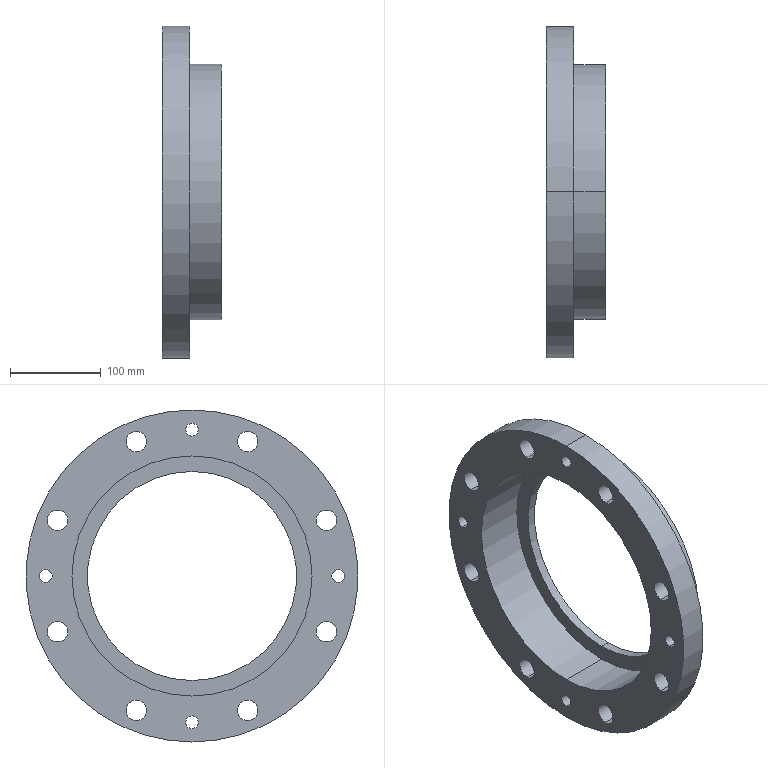Part | SolidWorks | features CirPattern 1, HoleWzd 1, ICE 1, RefAxis 1, Revolution 1 | 1 solid | 36 faces | box 65 x 365 x 365 mm | volume 1770977 mm3 | cylinder 32 | plane 4 | commonest cylinder face diameters 22.453 x16 14 x8 229.72 x2 264 x2 281 x2 365 x2
STEP:
#1=CARTESIAN_POINT('',(-49.177,0.,153.836));
#2=VERTEX_POINT('',#1);
#3=CARTESIAN_POINT('',(-49.177,0.,167.836));
#4=VERTEX_POINT('',#3);
#5=CARTESIAN_POINT('',(-49.177,0.,160.836));
#6=DIRECTION('',(-1.,0.,0.));
#7=DIRECTION('',(0.,0.,1.));
#8=AXIS2_PLACEMENT_3D('',#5,#6,#7);
#9=CIRCLE('',#8,7.);
#10=EDGE_CURVE('',#2,#4,#9,.T.);
#11=ORIENTED_EDGE('',*,*,#10,.F.);
#12=CARTESIAN_POINT('',(-79.177,0.,153.836));
#13=VERTEX_POINT('',#12);
#14=CARTESIAN_POINT('',(-79.177,0.,153.836));
#15=DIRECTION('',(-1.,0.,0.));
#16=VECTOR('',#15,1000.);
#17=LINE('',#14,#16);
#18=EDGE_CURVE('',#2,#13,#17,.T.);
#19=ORIENTED_EDGE('',*,*,#18,.T.);
#20=CARTESIAN_POINT('',(-79.177,0.,167.836));
#21=VERTEX_POINT('',#20);
#22=CARTESIAN_POINT('',(-79.177,0.,160.836));
#23=DIRECTION('',(-1.,0.,0.));
#24=DIRECTION('',(0.,0.,1.));
#25=AXIS2_PLACEMENT_3D('',#22,#23,#24);
#26=CIRCLE('',#25,7.);
#27=EDGE_CURVE('',#13,#21,#26,.T.);
#28=ORIENTED_EDGE('',*,*,#27,.T.);
#29=CARTESIAN_POINT('',(-79.177,0.,167.836));
#30=DIRECTION('',(-1.,0.,0.));
#31=VECTOR('',#30,1000.);
#32=LINE('',#29,#31);
#33=EDGE_CURVE('',#4,#21,#32,.T.);
#34=ORIENTED_EDGE('',*,*,#33,.F.);
#35=EDGE_LOOP('',(#11,#19,#28,#34));
#36=FACE_OUTER_BOUND('',#35,.T.);
#37=CARTESIAN_POINT('',(-79.177,0.,160.836));
#38=DIRECTION('',(-1.,0.,0.));
#39=DIRECTION('',(0.,0.,1.));
#40=AXIS2_PLACEMENT_3D('',#37,#38,#39);
#41=CYLINDRICAL_SURFACE('',#40,7.);
#42=ADVANCED_FACE('',(#36),#41,.F.);
#43=CARTESIAN_POINT('',(-49.177,-160.836,-7.));
#44=VERTEX_POINT('',#43);
#45=CARTESIAN_POINT('',(-49.177,-160.836,7.));
#46=VERTEX_POINT('',#45);
#47=CARTESIAN_POINT('',(-49.177,-160.836,0.));
#48=DIRECTION('',(-1.,0.,0.));
#49=DIRECTION('',(0.,0.,1.));
#50=AXIS2_PLACEMENT_3D('',#47,#48,#49);
#51=CIRCLE('',#50,7.);
#52=EDGE_CURVE('',#44,#46,#51,.T.);
#53=ORIENTED_EDGE('',*,*,#52,.F.);
#54=CARTESIAN_POINT('',(-79.177,-160.836,-7.));
#55=VERTEX_POINT('',#54);
#56=CARTESIAN_POINT('',(-79.177,-160.836,-7.));
#57=DIRECTION('',(-1.,0.,0.));
#58=VECTOR('',#57,1000.);
#59=LINE('',#56,#58);
#60=EDGE_CURVE('',#44,#55,#59,.T.);
#61=ORIENTED_EDGE('',*,*,#60,.T.);
#62=CARTESIAN_POINT('',(-79.177,-160.836,7.));
#63=VERTEX_POINT('',#62);
#64=CARTESIAN_POINT('',(-79.177,-160.836,0.));
#65=DIRECTION('',(-1.,0.,0.));
#66=DIRECTION('',(0.,0.,1.));
#67=AXIS2_PLACEMENT_3D('',#64,#65,#66);
#68=CIRCLE('',#67,7.);
#69=EDGE_CURVE('',#55,#63,#68,.T.);
#70=ORIENTED_EDGE('',*,*,#69,.T.);
#71=CARTESIAN_POINT('',(-79.177,-160.836,7.));
#72=DIRECTION('',(-1.,0.,0.));
#73=VECTOR('',#72,1000.);
#74=LINE('',#71,#73);
#75=EDGE_CURVE('',#46,#63,#74,.T.);
#76=ORIENTED_EDGE('',*,*,#75,.F.);
#77=EDGE_LOOP('',(#53,#61,#70,#76));
#78=FACE_OUTER_BOUND('',#77,.T.);
#79=CARTESIAN_POINT('',(-79.177,-160.836,0.));
#80=DIRECTION('',(-1.,0.,0.));
#81=DIRECTION('',(0.,0.,1.));
#82=AXIS2_PLACEMENT_3D('',#79,#80,#81);
#83=CYLINDRICAL_SURFACE('',#82,7.);
#84=ADVANCED_FACE('',(#78),#83,.F.);
#85=CARTESIAN_POINT('',(-49.177,0.,-167.836));
#86=VERTEX_POINT('',#85);
#87=CARTESIAN_POINT('',(-49.177,0.,-153.836));
#88=VERTEX_POINT('',#87);
#89=CARTESIAN_POINT('',(-49.177,0.,-160.836));
#90=DIRECTION('',(-1.,0.,0.));
#91=DIRECTION('',(0.,0.,1.));
#92=AXIS2_PLACEMENT_3D('',#89,#90,#91);
#93=CIRCLE('',#92,7.);
#94=EDGE_CURVE('',#86,#88,#93,.T.);
#95=ORIENTED_EDGE('',*,*,#94,.F.);
#96=CARTESIAN_POINT('',(-79.177,0.,-167.836));
#97=VERTEX_POINT('',#96);
#98=CARTESIAN_POINT('',(-79.177,0.,-167.836));
#99=DIRECTION('',(-1.,0.,0.));
#100=VECTOR('',#99,1000.);
#101=LINE('',#98,#100);
#102=EDGE_CURVE('',#86,#97,#101,.T.);
#103=ORIENTED_EDGE('',*,*,#102,.T.);
#104=CARTESIAN_POINT('',(-79.177,0.,-153.836));
#105=VERTEX_POINT('',#104);
#106=CARTESIAN_POINT('',(-79.177,0.,-160.836));
#107=DIRECTION('',(-1.,0.,0.));
#108=DIRECTION('',(0.,0.,1.));
#109=AXIS2_PLACEMENT_3D('',#106,#107,#108);
#110=CIRCLE('',#109,7.);
#111=EDGE_CURVE('',#97,#105,#110,.T.);
#112=ORIENTED_EDGE('',*,*,#111,.T.);
#113=CARTESIAN_POINT('',(-79.177,0.,-153.836));
#114=DIRECTION('',(-1.,0.,0.));
#115=VECTOR('',#114,1000.);
#116=LINE('',#113,#115);
#117=EDGE_CURVE('',#88,#105,#116,.T.);
#118=ORIENTED_EDGE('',*,*,#117,.F.);
#119=EDGE_LOOP('',(#95,#103,#112,#118));
#120=FACE_OUTER_BOUND('',#119,.T.);
#121=CARTESIAN_POINT('',(-79.177,0.,-160.836));
#122=DIRECTION('',(-1.,0.,0.));
#123=DIRECTION('',(0.,0.,1.));
#124=AXIS2_PLACEMENT_3D('',#121,#122,#123);
#125=CYLINDRICAL_SURFACE('',#124,7.);
#126=ADVANCED_FACE('',(#120),#125,.F.);
#127=CARTESIAN_POINT('',(-49.177,160.836,-7.));
#128=VERTEX_POINT('',#127);
#129=CARTESIAN_POINT('',(-49.177,160.836,7.));
#130=VERTEX_POINT('',#129);
#131=CARTESIAN_POINT('',(-49.177,160.836,0.));
#132=DIRECTION('',(-1.,0.,0.));
#133=DIRECTION('',(0.,0.,1.));
#134=AXIS2_PLACEMENT_3D('',#131,#132,#133);
#135=CIRCLE('',#134,7.);
#136=EDGE_CURVE('',#128,#130,#135,.T.);
#137=ORIENTED_EDGE('',*,*,#136,.F.);
#138=CARTESIAN_POINT('',(-79.177,160.836,-7.));
#139=VERTEX_POINT('',#138);
#140=CARTESIAN_POINT('',(-79.177,160.836,-7.));
#141=DIRECTION('',(-1.,0.,0.));
#142=VECTOR('',#141,1000.);
#143=LINE('',#140,#142);
#144=EDGE_CURVE('',#128,#139,#143,.T.);
#145=ORIENTED_EDGE('',*,*,#144,.T.);
#146=CARTESIAN_POINT('',(-79.177,160.836,7.));
#147=VERTEX_POINT('',#146);
#148=CARTESIAN_POINT('',(-79.177,160.836,0.));
#149=DIRECTION('',(-1.,0.,0.));
#150=DIRECTION('',(0.,0.,1.));
#151=AXIS2_PLACEMENT_3D('',#148,#149,#150);
#152=CIRCLE('',#151,7.);
#153=EDGE_CURVE('',#139,#147,#152,.T.);
#154=ORIENTED_EDGE('',*,*,#153,.T.);
#155=CARTESIAN_POINT('',(-79.177,160.836,7.));
#156=DIRECTION('',(-1.,0.,0.));
#157=VECTOR('',#156,1000.);
#158=LINE('',#155,#157);
#159=EDGE_CURVE('',#130,#147,#158,.T.);
#160=ORIENTED_EDGE('',*,*,#159,.F.);
#161=EDGE_LOOP('',(#137,#145,#154,#160));
#162=FACE_OUTER_BOUND('',#161,.T.);
#163=CARTESIAN_POINT('',(-79.177,160.836,0.));
#164=DIRECTION('',(-1.,0.,0.));
#165=DIRECTION('',(0.,0.,1.));
#166=AXIS2_PLACEMENT_3D('',#163,#164,#165);
#167=CYLINDRICAL_SURFACE('',#166,7.);
#168=ADVANCED_FACE('',(#162),#167,.F.);
#169=CARTESIAN_POINT('',(-49.177,147.821,-72.456));
#170=VERTEX_POINT('',#169);
#171=CARTESIAN_POINT('',(-49.177,147.821,-50.003));
#172=VERTEX_POINT('',#171);
#173=CARTESIAN_POINT('',(-49.177,147.821,-61.229));
#174=DIRECTION('',(-1.,0.,0.));
#175=DIRECTION('',(0.,0.,1.));
#176=AXIS2_PLACEMENT_3D('',#173,#174,#175);
#177=CIRCLE('',#176,11.227);
#178=EDGE_CURVE('',#170,#172,#177,.T.);
#179=ORIENTED_EDGE('',*,*,#178,.F.);
#180=CARTESIAN_POINT('',(-79.177,147.821,-72.456));
#181=VERTEX_POINT('',#180);
#182=CARTESIAN_POINT('',(-49.177,147.821,-72.456));
#183=DIRECTION('',(-1.,0.,0.));
#184=VECTOR('',#183,1000.);
#185=LINE('',#182,#184);
#186=EDGE_CURVE('',#170,#181,#185,.T.);
#187=ORIENTED_EDGE('',*,*,#186,.T.);
#188=CARTESIAN_POINT('',(-79.177,147.821,-50.003));
#189=VERTEX_POINT('',#188);
#190=CARTESIAN_POINT('',(-79.177,147.821,-61.229));
#191=DIRECTION('',(-1.,0.,0.));
#192=DIRECTION('',(0.,0.,1.));
#193=AXIS2_PLACEMENT_3D('',#190,#191,#192);
#194=CIRCLE('',#193,11.227);
#195=EDGE_CURVE('',#181,#189,#194,.T.);
#196=ORIENTED_EDGE('',*,*,#195,.T.);
#197=CARTESIAN_POINT('',(-49.177,147.821,-50.003));
#198=DIRECTION('',(-1.,0.,0.));
#199=VECTOR('',#198,1000.);
#200=LINE('',#197,#199);
#201=EDGE_CURVE('',#172,#189,#200,.T.);
#202=ORIENTED_EDGE('',*,*,#201,.F.);
#203=EDGE_LOOP('',(#179,#187,#196,#202));
#204=FACE_OUTER_BOUND('',#203,.T.);
#205=CARTESIAN_POINT('',(-49.177,147.821,-61.229));
#206=DIRECTION('',(-1.,0.,0.));
#207=DIRECTION('',(0.,0.,1.));
#208=AXIS2_PLACEMENT_3D('',#205,#206,#207);
#209=CYLINDRICAL_SURFACE('',#208,11.227);
#210=ADVANCED_FACE('',(#204),#209,.F.);
#211=CARTESIAN_POINT('',(-49.177,61.229,-159.047));
#212=VERTEX_POINT('',#211);
#213=CARTESIAN_POINT('',(-49.177,61.229,-136.594));
#214=VERTEX_POINT('',#213);
#215=CARTESIAN_POINT('',(-49.177,61.229,-147.821));
#216=DIRECTION('',(-1.,0.,0.));
#217=DIRECTION('',(0.,0.,1.));
#218=AXIS2_PLACEMENT_3D('',#215,#216,#217);
#219=CIRCLE('',#218,11.227);
#220=EDGE_CURVE('',#212,#214,#219,.T.);
#221=ORIENTED_EDGE('',*,*,#220,.F.);
#222=CARTESIAN_POINT('',(-79.177,61.229,-159.047));
#223=VERTEX_POINT('',#222);
#224=CARTESIAN_POINT('',(-49.177,61.229,-159.047));
#225=DIRECTION('',(-1.,0.,0.));
#226=VECTOR('',#225,1000.);
#227=LINE('',#224,#226);
#228=EDGE_CURVE('',#212,#223,#227,.T.);
#229=ORIENTED_EDGE('',*,*,#228,.T.);
#230=CARTESIAN_POINT('',(-79.177,61.229,-136.594));
#231=VERTEX_POINT('',#230);
#232=CARTESIAN_POINT('',(-79.177,61.229,-147.821));
#233=DIRECTION('',(-1.,0.,0.));
#234=DIRECTION('',(0.,0.,1.));
#235=AXIS2_PLACEMENT_3D('',#232,#233,#234);
#236=CIRCLE('',#235,11.227);
#237=EDGE_CURVE('',#223,#231,#236,.T.);
#238=ORIENTED_EDGE('',*,*,#237,.T.);
#239=CARTESIAN_POINT('',(-49.177,61.229,-136.594));
#240=DIRECTION('',(-1.,0.,0.));
#241=VECTOR('',#240,1000.);
#242=LINE('',#239,#241);
#243=EDGE_CURVE('',#214,#231,#242,.T.);
#244=ORIENTED_EDGE('',*,*,#243,.F.);
#245=EDGE_LOOP('',(#221,#229,#238,#244));
#246=FACE_OUTER_BOUND('',#245,.T.);
#247=CARTESIAN_POINT('',(-49.177,61.229,-147.821));
#248=DIRECTION('',(-1.,0.,0.));
#249=DIRECTION('',(0.,0.,1.));
#250=AXIS2_PLACEMENT_3D('',#247,#248,#249);
#251=CYLINDRICAL_SURFACE('',#250,11.227);
#252=ADVANCED_FACE('',(#246),#251,.F.);
#253=CARTESIAN_POINT('',(-49.177,-61.229,-159.047));
#254=VERTEX_POINT('',#253);
#255=CARTESIAN_POINT('',(-49.177,-61.229,-136.594));
#256=VERTEX_POINT('',#255);
#257=CARTESIAN_POINT('',(-49.177,-61.229,-147.821));
#258=DIRECTION('',(-1.,0.,0.));
#259=DIRECTION('',(0.,0.,1.));
#260=AXIS2_PLACEMENT_3D('',#257,#258,#259);
#261=CIRCLE('',#260,11.227);
#262=EDGE_CURVE('',#254,#256,#261,.T.);
#263=ORIENTED_EDGE('',*,*,#262,.F.);
#264=CARTESIAN_POINT('',(-79.177,-61.229,-159.047));
#265=VERTEX_POINT('',#264);
#266=CARTESIAN_POINT('',(-49.177,-61.229,-159.047));
#267=DIRECTION('',(-1.,0.,0.));
#268=VECTOR('',#267,1000.);
#269=LINE('',#266,#268);
#270=EDGE_CURVE('',#254,#265,#269,.T.);
#271=ORIENTED_EDGE('',*,*,#270,.T.);
#272=CARTESIAN_POINT('',(-79.177,-61.229,-136.594));
#273=VERTEX_POINT('',#272);
#274=CARTESIAN_POINT('',(-79.177,-61.229,-147.821));
#275=DIRECTION('',(-1.,0.,0.));
#276=DIRECTION('',(0.,0.,1.));
#277=AXIS2_PLACEMENT_3D('',#274,#275,#276);
#278=CIRCLE('',#277,11.227);
#279=EDGE_CURVE('',#265,#273,#278,.T.);
#280=ORIENTED_EDGE('',*,*,#279,.T.);
#281=CARTESIAN_POINT('',(-49.177,-61.229,-136.594));
#282=DIRECTION('',(-1.,0.,0.));
#283=VECTOR('',#282,1000.);
#284=LINE('',#281,#283);
#285=EDGE_CURVE('',#256,#273,#284,.T.);
#286=ORIENTED_EDGE('',*,*,#285,.F.);
#287=EDGE_LOOP('',(#263,#271,#280,#286));
#288=FACE_OUTER_BOUND('',#287,.T.);
#289=CARTESIAN_POINT('',(-49.177,-61.229,-147.821));
#290=DIRECTION('',(-1.,0.,0.));
#291=DIRECTION('',(0.,0.,1.));
#292=AXIS2_PLACEMENT_3D('',#289,#290,#291);
#293=CYLINDRICAL_SURFACE('',#292,11.227);
#294=ADVANCED_FACE('',(#288),#293,.F.);
#295=CARTESIAN_POINT('',(-49.177,-147.821,-72.456));
#296=VERTEX_POINT('',#295);
#297=CARTESIAN_POINT('',(-49.177,-147.821,-50.003));
#298=VERTEX_POINT('',#297);
#299=CARTESIAN_POINT('',(-49.177,-147.821,-61.229));
#300=DIRECTION('',(-1.,0.,0.));
#301=DIRECTION('',(0.,0.,1.));
#302=AXIS2_PLACEMENT_3D('',#299,#300,#301);
#303=CIRCLE('',#302,11.227);
#304=EDGE_CURVE('',#296,#298,#303,.T.);
#305=ORIENTED_EDGE('',*,*,#304,.F.);
#306=CARTESIAN_POINT('',(-79.177,-147.821,-72.456));
#307=VERTEX_POINT('',#306);
#308=CARTESIAN_POINT('',(-49.177,-147.821,-72.456));
#309=DIRECTION('',(-1.,0.,0.));
#310=VECTOR('',#309,1000.);
#311=LINE('',#308,#310);
#312=EDGE_CURVE('',#296,#307,#311,.T.);
#313=ORIENTED_EDGE('',*,*,#312,.T.);
#314=CARTESIAN_POINT('',(-79.177,-147.821,-50.003));
#315=VERTEX_POINT('',#314);
#316=CARTESIAN_POINT('',(-79.177,-147.821,-61.229));
#317=DIRECTION('',(-1.,0.,0.));
#318=DIRECTION('',(0.,0.,1.));
#319=AXIS2_PLACEMENT_3D('',#316,#317,#318);
#320=CIRCLE('',#319,11.227);
#321=EDGE_CURVE('',#307,#315,#320,.T.);
#322=ORIENTED_EDGE('',*,*,#321,.T.);
#323=CARTESIAN_POINT('',(-49.177,-147.821,-50.003));
#324=DIRECTION('',(-1.,0.,0.));
#325=VECTOR('',#324,1000.);
#326=LINE('',#323,#325);
#327=EDGE_CURVE('',#298,#315,#326,.T.);
#328=ORIENTED_EDGE('',*,*,#327,.F.);
#329=EDGE_LOOP('',(#305,#313,#322,#328));
#330=FACE_OUTER_BOUND('',#329,.T.);
#331=CARTESIAN_POINT('',(-49.177,-147.821,-61.229));
#332=DIRECTION('',(-1.,0.,0.));
#333=DIRECTION('',(0.,0.,1.));
#334=AXIS2_PLACEMENT_3D('',#331,#332,#333);
#335=CYLINDRICAL_SURFACE('',#334,11.227);
#336=ADVANCED_FACE('',(#330),#335,.F.);
#337=CARTESIAN_POINT('',(-49.177,-147.821,50.003));
#338=VERTEX_POINT('',#337);
#339=CARTESIAN_POINT('',(-49.177,-147.821,72.456));
#340=VERTEX_POINT('',#339);
#341=CARTESIAN_POINT('',(-49.177,-147.821,61.229));
#342=DIRECTION('',(-1.,0.,0.));
#343=DIRECTION('',(0.,0.,1.));
#344=AXIS2_PLACEMENT_3D('',#341,#342,#343);
#345=CIRCLE('',#344,11.227);
#346=EDGE_CURVE('',#338,#340,#345,.T.);
#347=ORIENTED_EDGE('',*,*,#346,.F.);
#348=CARTESIAN_POINT('',(-79.177,-147.821,50.003));
#349=VERTEX_POINT('',#348);
#350=CARTESIAN_POINT('',(-49.177,-147.821,50.003));
#351=DIRECTION('',(-1.,0.,0.));
#352=VECTOR('',#351,1000.);
#353=LINE('',#350,#352);
#354=EDGE_CURVE('',#338,#349,#353,.T.);
#355=ORIENTED_EDGE('',*,*,#354,.T.);
#356=CARTESIAN_POINT('',(-79.177,-147.821,72.456));
#357=VERTEX_POINT('',#356);
#358=CARTESIAN_POINT('',(-79.177,-147.821,61.229));
#359=DIRECTION('',(-1.,0.,0.));
#360=DIRECTION('',(0.,0.,1.));
#361=AXIS2_PLACEMENT_3D('',#358,#359,#360);
#362=CIRCLE('',#361,11.227);
#363=EDGE_CURVE('',#349,#357,#362,.T.);
#364=ORIENTED_EDGE('',*,*,#363,.T.);
#365=CARTESIAN_POINT('',(-49.177,-147.821,72.456));
#366=DIRECTION('',(-1.,0.,0.));
#367=VECTOR('',#366,1000.);
#368=LINE('',#365,#367);
#369=EDGE_CURVE('',#340,#357,#368,.T.);
#370=ORIENTED_EDGE('',*,*,#369,.F.);
#371=EDGE_LOOP('',(#347,#355,#364,#370));
#372=FACE_OUTER_BOUND('',#371,.T.);
#373=CARTESIAN_POINT('',(-49.177,-147.821,61.229));
#374=DIRECTION('',(-1.,0.,0.));
#375=DIRECTION('',(0.,0.,1.));
#376=AXIS2_PLACEMENT_3D('',#373,#374,#375);
#377=CYLINDRICAL_SURFACE('',#376,11.227);
#378=ADVANCED_FACE('',(#372),#377,.F.);
#379=CARTESIAN_POINT('',(-49.177,-61.229,136.594));
#380=VERTEX_POINT('',#379);
#381=CARTESIAN_POINT('',(-49.177,-61.229,159.047));
#382=VERTEX_POINT('',#381);
#383=CARTESIAN_POINT('',(-49.177,-61.229,147.821));
#384=DIRECTION('',(-1.,0.,0.));
#385=DIRECTION('',(0.,0.,1.));
#386=AXIS2_PLACEMENT_3D('',#383,#384,#385);
#387=CIRCLE('',#386,11.227);
#388=EDGE_CURVE('',#380,#382,#387,.T.);
#389=ORIENTED_EDGE('',*,*,#388,.F.);
#390=CARTESIAN_POINT('',(-79.177,-61.229,136.594));
#391=VERTEX_POINT('',#390);
#392=CARTESIAN_POINT('',(-49.177,-61.229,136.594));
#393=DIRECTION('',(-1.,0.,0.));
#394=VECTOR('',#393,1000.);
#395=LINE('',#392,#394);
#396=EDGE_CURVE('',#380,#391,#395,.T.);
#397=ORIENTED_EDGE('',*,*,#396,.T.);
#398=CARTESIAN_POINT('',(-79.177,-61.229,159.047));
#399=VERTEX_POINT('',#398);
#400=CARTESIAN_POINT('',(-79.177,-61.229,147.821));
#401=DIRECTION('',(-1.,0.,0.));
#402=DIRECTION('',(0.,0.,1.));
#403=AXIS2_PLACEMENT_3D('',#400,#401,#402);
#404=CIRCLE('',#403,11.227);
#405=EDGE_CURVE('',#391,#399,#404,.T.);
#406=ORIENTED_EDGE('',*,*,#405,.T.);
#407=CARTESIAN_POINT('',(-49.177,-61.229,159.047));
#408=DIRECTION('',(-1.,0.,0.));
#409=VECTOR('',#408,1000.);
#410=LINE('',#407,#409);
#411=EDGE_CURVE('',#382,#399,#410,.T.);
#412=ORIENTED_EDGE('',*,*,#411,.F.);
#413=EDGE_LOOP('',(#389,#397,#406,#412));
#414=FACE_OUTER_BOUND('',#413,.T.);
#415=CARTESIAN_POINT('',(-49.177,-61.229,147.821));
#416=DIRECTION('',(-1.,0.,0.));
#417=DIRECTION('',(0.,0.,1.));
#418=AXIS2_PLACEMENT_3D('',#415,#416,#417);
#419=CYLINDRICAL_SURFACE('',#418,11.227);
#420=ADVANCED_FACE('',(#414),#419,.F.);
#421=CARTESIAN_POINT('',(-49.177,61.229,136.594));
#422=VERTEX_POINT('',#421);
#423=CARTESIAN_POINT('',(-49.177,61.229,159.047));
#424=VERTEX_POINT('',#423);
#425=CARTESIAN_POINT('',(-49.177,61.229,147.821));
#426=DIRECTION('',(-1.,0.,0.));
#427=DIRECTION('',(0.,0.,1.));
#428=AXIS2_PLACEMENT_3D('',#425,#426,#427);
#429=CIRCLE('',#428,11.227);
#430=EDGE_CURVE('',#422,#424,#429,.T.);
#431=ORIENTED_EDGE('',*,*,#430,.F.);
#432=CARTESIAN_POINT('',(-79.177,61.229,136.594));
#433=VERTEX_POINT('',#432);
#434=CARTESIAN_POINT('',(-49.177,61.229,136.594));
#435=DIRECTION('',(-1.,0.,0.));
#436=VECTOR('',#435,1000.);
#437=LINE('',#434,#436);
#438=EDGE_CURVE('',#422,#433,#437,.T.);
#439=ORIENTED_EDGE('',*,*,#438,.T.);
#440=CARTESIAN_POINT('',(-79.177,61.229,159.047));
#441=VERTEX_POINT('',#440);
#442=CARTESIAN_POINT('',(-79.177,61.229,147.821));
#443=DIRECTION('',(-1.,0.,0.));
#444=DIRECTION('',(0.,0.,1.));
#445=AXIS2_PLACEMENT_3D('',#442,#443,#444);
#446=CIRCLE('',#445,11.227);
#447=EDGE_CURVE('',#433,#441,#446,.T.);
#448=ORIENTED_EDGE('',*,*,#447,.T.);
#449=CARTESIAN_POINT('',(-49.177,61.229,159.047));
#450=DIRECTION('',(-1.,0.,0.));
#451=VECTOR('',#450,1000.);
#452=LINE('',#449,#451);
#453=EDGE_CURVE('',#424,#441,#452,.T.);
#454=ORIENTED_EDGE('',*,*,#453,.F.);
#455=EDGE_LOOP('',(#431,#439,#448,#454));
#456=FACE_OUTER_BOUND('',#455,.T.);
#457=CARTESIAN_POINT('',(-49.177,61.229,147.821));
#458=DIRECTION('',(-1.,0.,0.));
#459=DIRECTION('',(0.,0.,1.));
#460=AXIS2_PLACEMENT_3D('',#457,#458,#459);
#461=CYLINDRICAL_SURFACE('',#460,11.227);
#462=ADVANCED_FACE('',(#456),#461,.F.);
#463=CARTESIAN_POINT('',(-49.177,147.821,50.003));
#464=VERTEX_POINT('',#463);
#465=CARTESIAN_POINT('',(-49.177,147.821,72.456));
#466=VERTEX_POINT('',#465);
#467=CARTESIAN_POINT('',(-49.177,147.821,61.229));
#468=DIRECTION('',(-1.,0.,0.));
#469=DIRECTION('',(0.,0.,1.));
#470=AXIS2_PLACEMENT_3D('',#467,#468,#469);
#471=CIRCLE('',#470,11.227);
#472=EDGE_CURVE('',#464,#466,#471,.T.);
#473=ORIENTED_EDGE('',*,*,#472,.F.);
#474=CARTESIAN_POINT('',(-79.177,147.821,50.003));
#475=VERTEX_POINT('',#474);
#476=CARTESIAN_POINT('',(-49.177,147.821,50.003));
#477=DIRECTION('',(-1.,0.,0.));
#478=VECTOR('',#477,1000.);
#479=LINE('',#476,#478);
#480=EDGE_CURVE('',#464,#475,#479,.T.);
#481=ORIENTED_EDGE('',*,*,#480,.T.);
#482=CARTESIAN_POINT('',(-79.177,147.821,72.456));
#483=VERTEX_POINT('',#482);
#484=CARTESIAN_POINT('',(-79.177,147.821,61.229));
#485=DIRECTION('',(-1.,0.,0.));
#486=DIRECTION('',(0.,0.,1.));
#487=AXIS2_PLACEMENT_3D('',#484,#485,#486);
#488=CIRCLE('',#487,11.227);
#489=EDGE_CURVE('',#475,#483,#488,.T.);
#490=ORIENTED_EDGE('',*,*,#489,.T.);
#491=CARTESIAN_POINT('',(-49.177,147.821,72.456));
#492=DIRECTION('',(-1.,0.,0.));
#493=VECTOR('',#492,1000.);
#494=LINE('',#491,#493);
#495=EDGE_CURVE('',#466,#483,#494,.T.);
#496=ORIENTED_EDGE('',*,*,#495,.F.);
#497=EDGE_LOOP('',(#473,#481,#490,#496));
#498=FACE_OUTER_BOUND('',#497,.T.);
#499=CARTESIAN_POINT('',(-49.177,147.821,61.229));
#500=DIRECTION('',(-1.,0.,0.));
#501=DIRECTION('',(0.,0.,1.));
#502=AXIS2_PLACEMENT_3D('',#499,#500,#501);
#503=CYLINDRICAL_SURFACE('',#502,11.227);
#504=ADVANCED_FACE('',(#498),#503,.F.);
#505=CARTESIAN_POINT('',(-49.177,0.,182.5));
#506=VERTEX_POINT('',#505);
#507=CARTESIAN_POINT('',(-49.177,0.,-182.5));
#508=VERTEX_POINT('',#507);
#509=CARTESIAN_POINT('',(-49.177,0.,0.));
#510=DIRECTION('',(-1.,0.,0.));
#511=DIRECTION('',(0.,0.,1.));
#512=AXIS2_PLACEMENT_3D('',#509,#510,#511);
#513=CIRCLE('',#512,182.5);
#514=EDGE_CURVE('',#506,#508,#513,.T.);
#515=ORIENTED_EDGE('',*,*,#514,.T.);
#516=CARTESIAN_POINT('',(-79.177,0.,-182.5));
#517=VERTEX_POINT('',#516);
#518=CARTESIAN_POINT('',(-169.441,0.,-182.5));
#519=DIRECTION('',(-1.,0.,0.));
#520=VECTOR('',#519,1000.);
#521=LINE('',#518,#520);
#522=EDGE_CURVE('',#508,#517,#521,.T.);
#523=ORIENTED_EDGE('',*,*,#522,.T.);
#524=CARTESIAN_POINT('',(-79.177,0.,182.5));
#525=VERTEX_POINT('',#524);
#526=CARTESIAN_POINT('',(-79.177,0.,0.));
#527=DIRECTION('',(-1.,0.,0.));
#528=DIRECTION('',(0.,0.,1.));
#529=AXIS2_PLACEMENT_3D('',#526,#527,#528);
#530=CIRCLE('',#529,182.5);
#531=EDGE_CURVE('',#525,#517,#530,.T.);
#532=ORIENTED_EDGE('',*,*,#531,.F.);
#533=CARTESIAN_POINT('',(-169.441,0.,182.5));
#534=DIRECTION('',(-1.,0.,0.));
#535=VECTOR('',#534,1000.);
#536=LINE('',#533,#535);
#537=EDGE_CURVE('',#506,#525,#536,.T.);
#538=ORIENTED_EDGE('',*,*,#537,.F.);
#539=EDGE_LOOP('',(#515,#523,#532,#538));
#540=FACE_OUTER_BOUND('',#539,.T.);
#541=CARTESIAN_POINT('',(-169.441,0.,0.));
#542=DIRECTION('',(-1.,0.,0.));
#543=DIRECTION('',(0.,0.,1.));
#544=AXIS2_PLACEMENT_3D('',#541,#542,#543);
#545=CYLINDRICAL_SURFACE('',#544,182.5);
#546=ADVANCED_FACE('',(#540),#545,.T.);
#547=CARTESIAN_POINT('',(-14.177,0.,140.5));
#548=VERTEX_POINT('',#547);
#549=CARTESIAN_POINT('',(-14.177,0.,-140.5));
#550=VERTEX_POINT('',#549);
#551=CARTESIAN_POINT('',(-14.177,0.,0.));
#552=DIRECTION('',(-1.,0.,0.));
#553=DIRECTION('',(0.,0.,1.));
#554=AXIS2_PLACEMENT_3D('',#551,#552,#553);
#555=CIRCLE('',#554,140.5);
#556=EDGE_CURVE('',#548,#550,#555,.T.);
#557=ORIENTED_EDGE('',*,*,#556,.T.);
#558=CARTESIAN_POINT('',(-49.177,0.,-140.5));
#559=VERTEX_POINT('',#558);
#560=CARTESIAN_POINT('',(-169.441,0.,-140.5));
#561=DIRECTION('',(-1.,0.,0.));
#562=VECTOR('',#561,1000.);
#563=LINE('',#560,#562);
#564=EDGE_CURVE('',#550,#559,#563,.T.);
#565=ORIENTED_EDGE('',*,*,#564,.T.);
#566=CARTESIAN_POINT('',(-49.177,0.,140.5));
#567=VERTEX_POINT('',#566);
#568=CARTESIAN_POINT('',(-49.177,0.,0.));
#569=DIRECTION('',(-1.,0.,0.));
#570=DIRECTION('',(0.,0.,1.));
#571=AXIS2_PLACEMENT_3D('',#568,#569,#570);
#572=CIRCLE('',#571,140.5);
#573=EDGE_CURVE('',#567,#559,#572,.T.);
#574=ORIENTED_EDGE('',*,*,#573,.F.);
#575=CARTESIAN_POINT('',(-169.441,0.,140.5));
#576=DIRECTION('',(-1.,0.,0.));
#577=VECTOR('',#576,1000.);
#578=LINE('',#575,#577);
#579=EDGE_CURVE('',#548,#567,#578,.T.);
#580=ORIENTED_EDGE('',*,*,#579,.F.);
#581=EDGE_LOOP('',(#557,#565,#574,#580));
#582=FACE_OUTER_BOUND('',#581,.T.);
#583=CARTESIAN_POINT('',(-169.441,0.,0.));
#584=DIRECTION('',(-1.,0.,0.));
#585=DIRECTION('',(0.,0.,1.));
#586=AXIS2_PLACEMENT_3D('',#583,#584,#585);
#587=CYLINDRICAL_SURFACE('',#586,140.5);
#588=ADVANCED_FACE('',(#582),#587,.T.);
#589=CARTESIAN_POINT('',(-14.177,0.,-114.86));
#590=VERTEX_POINT('',#589);
#591=CARTESIAN_POINT('',(-14.177,0.,114.86));
#592=VERTEX_POINT('',#591);
#593=CARTESIAN_POINT('',(-14.177,0.,0.));
#594=DIRECTION('',(-1.,0.,0.));
#595=DIRECTION('',(0.,0.,1.));
#596=AXIS2_PLACEMENT_3D('',#593,#594,#595);
#597=CIRCLE('',#596,114.86);
#598=EDGE_CURVE('',#590,#592,#597,.T.);
#599=ORIENTED_EDGE('',*,*,#598,.F.);
#600=CARTESIAN_POINT('',(-24.177,0.,-114.86));
#601=VERTEX_POINT('',#600);
#602=CARTESIAN_POINT('',(-169.441,0.,-114.86));
#603=DIRECTION('',(-1.,0.,0.));
#604=VECTOR('',#603,1000.);
#605=LINE('',#602,#604);
#606=EDGE_CURVE('',#590,#601,#605,.T.);
#607=ORIENTED_EDGE('',*,*,#606,.T.);
#608=CARTESIAN_POINT('',(-24.177,0.,114.86));
#609=VERTEX_POINT('',#608);
#610=CARTESIAN_POINT('',(-24.177,0.,0.));
#611=DIRECTION('',(-1.,0.,0.));
#612=DIRECTION('',(0.,0.,1.));
#613=AXIS2_PLACEMENT_3D('',#610,#611,#612);
#614=CIRCLE('',#613,114.86);
#615=EDGE_CURVE('',#601,#609,#614,.T.);
#616=ORIENTED_EDGE('',*,*,#615,.T.);
#617=CARTESIAN_POINT('',(-169.441,0.,114.86));
#618=DIRECTION('',(-1.,0.,0.));
#619=VECTOR('',#618,1000.);
#620=LINE('',#617,#619);
#621=EDGE_CURVE('',#592,#609,#620,.T.);
#622=ORIENTED_EDGE('',*,*,#621,.F.);
#623=EDGE_LOOP('',(#599,#607,#616,#622));
#624=FACE_OUTER_BOUND('',#623,.T.);
#625=CARTESIAN_POINT('',(-169.441,0.,0.));
#626=DIRECTION('',(-1.,0.,0.));
#627=DIRECTION('',(0.,0.,1.));
#628=AXIS2_PLACEMENT_3D('',#625,#626,#627);
#629=CYLINDRICAL_SURFACE('',#628,114.86);
#630=ADVANCED_FACE('',(#624),#629,.F.);
#631=CARTESIAN_POINT('',(-24.177,0.,-132.));
#632=VERTEX_POINT('',#631);
#633=CARTESIAN_POINT('',(-24.177,0.,132.));
#634=VERTEX_POINT('',#633);
#635=CARTESIAN_POINT('',(-24.177,0.,0.));
#636=DIRECTION('',(-1.,0.,0.));
#637=DIRECTION('',(0.,0.,1.));
#638=AXIS2_PLACEMENT_3D('',#635,#636,#637);
#639=CIRCLE('',#638,132.);
#640=EDGE_CURVE('',#632,#634,#639,.T.);
#641=ORIENTED_EDGE('',*,*,#640,.F.);
#642=CARTESIAN_POINT('',(-79.177,0.,-132.));
#643=VERTEX_POINT('',#642);
#644=CARTESIAN_POINT('',(-169.441,0.,-132.));
#645=DIRECTION('',(-1.,0.,0.));
#646=VECTOR('',#645,1000.);
#647=LINE('',#644,#646);
#648=EDGE_CURVE('',#632,#643,#647,.T.);
#649=ORIENTED_EDGE('',*,*,#648,.T.);
#650=CARTESIAN_POINT('',(-79.177,0.,132.));
#651=VERTEX_POINT('',#650);
#652=CARTESIAN_POINT('',(-79.177,0.,0.));
#653=DIRECTION('',(-1.,0.,0.));
#654=DIRECTION('',(0.,0.,1.));
#655=AXIS2_PLACEMENT_3D('',#652,#653,#654);
#656=CIRCLE('',#655,132.);
#657=EDGE_CURVE('',#643,#651,#656,.T.);
#658=ORIENTED_EDGE('',*,*,#657,.T.);
#659=CARTESIAN_POINT('',(-169.441,0.,132.));
#660=DIRECTION('',(-1.,0.,0.));
#661=VECTOR('',#660,1000.);
#662=LINE('',#659,#661);
#663=EDGE_CURVE('',#634,#651,#662,.T.);
#664=ORIENTED_EDGE('',*,*,#663,.F.);
#665=EDGE_LOOP('',(#641,#649,#658,#664));
#666=FACE_OUTER_BOUND('',#665,.T.);
#667=CARTESIAN_POINT('',(-169.441,0.,0.));
#668=DIRECTION('',(-1.,0.,0.));
#669=DIRECTION('',(0.,0.,1.));
#670=AXIS2_PLACEMENT_3D('',#667,#668,#669);
#671=CYLINDRICAL_SURFACE('',#670,132.);
#672=ADVANCED_FACE('',(#666),#671,.F.);
#673=ORIENTED_EDGE('',*,*,#648,.F.);
#674=CARTESIAN_POINT('',(-24.177,0.,0.));
#675=DIRECTION('',(-1.,0.,0.));
#676=DIRECTION('',(0.,0.,1.));
#677=AXIS2_PLACEMENT_3D('',#674,#675,#676);
#678=CIRCLE('',#677,132.);
#679=EDGE_CURVE('',#634,#632,#678,.T.);
#680=ORIENTED_EDGE('',*,*,#679,.F.);
#681=ORIENTED_EDGE('',*,*,#663,.T.);
#682=CARTESIAN_POINT('',(-79.177,0.,0.));
#683=DIRECTION('',(-1.,0.,0.));
#684=DIRECTION('',(0.,0.,1.));
#685=AXIS2_PLACEMENT_3D('',#682,#683,#684);
#686=CIRCLE('',#685,132.);
#687=EDGE_CURVE('',#651,#643,#686,.T.);
#688=ORIENTED_EDGE('',*,*,#687,.T.);
#689=EDGE_LOOP('',(#673,#680,#681,#688));
#690=FACE_OUTER_BOUND('',#689,.T.);
#691=CARTESIAN_POINT('',(-169.441,0.,0.));
#692=DIRECTION('',(-1.,0.,0.));
#693=DIRECTION('',(0.,0.,1.));
#694=AXIS2_PLACEMENT_3D('',#691,#692,#693);
#695=CYLINDRICAL_SURFACE('',#694,132.);
#696=ADVANCED_FACE('',(#690),#695,.F.);
#697=CARTESIAN_POINT('',(-24.177,0.,0.));
#698=DIRECTION('',(-1.,0.,0.));
#699=DIRECTION('',(0.,0.,1.));
#700=AXIS2_PLACEMENT_3D('',#697,#698,#699);
#701=CIRCLE('',#700,114.86);
#702=EDGE_CURVE('',#609,#601,#701,.T.);
#703=ORIENTED_EDGE('',*,*,#702,.F.);
#704=ORIENTED_EDGE('',*,*,#615,.F.);
#705=EDGE_LOOP('',(#703,#704));
#706=FACE_BOUND('',#705,.T.);
#707=ORIENTED_EDGE('',*,*,#679,.T.);
#708=ORIENTED_EDGE('',*,*,#640,.T.);
#709=EDGE_LOOP('',(#707,#708));
#710=FACE_OUTER_BOUND('',#709,.T.);
#711=CARTESIAN_POINT('',(-24.177,114.86,0.));
#712=DIRECTION('',(1.,0.,0.));
#713=DIRECTION('',(0.,0.,-1.));
#714=AXIS2_PLACEMENT_3D('',#711,#712,#713);
#715=PLANE('',#714);
#716=ADVANCED_FACE('',(#706,#710),#715,.F.);
#717=ORIENTED_EDGE('',*,*,#606,.F.);
#718=CARTESIAN_POINT('',(-14.177,0.,0.));
#719=DIRECTION('',(-1.,0.,0.));
#720=DIRECTION('',(0.,0.,1.));
#721=AXIS2_PLACEMENT_3D('',#718,#719,#720);
#722=CIRCLE('',#721,114.86);
#723=EDGE_CURVE('',#592,#590,#722,.T.);
#724=ORIENTED_EDGE('',*,*,#723,.F.);
#725=ORIENTED_EDGE('',*,*,#621,.T.);
#726=ORIENTED_EDGE('',*,*,#702,.T.);
#727=EDGE_LOOP('',(#717,#724,#725,#726));
#728=FACE_OUTER_BOUND('',#727,.T.);
#729=CARTESIAN_POINT('',(-169.441,0.,0.));
#730=DIRECTION('',(-1.,0.,0.));
#731=DIRECTION('',(0.,0.,1.));
#732=AXIS2_PLACEMENT_3D('',#729,#730,#731);
#733=CYLINDRICAL_SURFACE('',#732,114.86);
#734=ADVANCED_FACE('',(#728),#733,.F.);
#735=ORIENTED_EDGE('',*,*,#556,.F.);
#736=CARTESIAN_POINT('',(-14.177,0.,0.));
#737=DIRECTION('',(-1.,0.,0.));
#738=DIRECTION('',(0.,0.,1.));
#739=AXIS2_PLACEMENT_3D('',#736,#737,#738);
#740=CIRCLE('',#739,140.5);
#741=EDGE_CURVE('',#550,#548,#740,.T.);
#742=ORIENTED_EDGE('',*,*,#741,.F.);
#743=EDGE_LOOP('',(#735,#742));
#744=FACE_OUTER_BOUND('',#743,.T.);
#745=ORIENTED_EDGE('',*,*,#723,.T.);
#746=ORIENTED_EDGE('',*,*,#598,.T.);
#747=EDGE_LOOP('',(#745,#746));
#748=FACE_BOUND('',#747,.T.);
#749=CARTESIAN_POINT('',(-14.177,140.5,0.));
#750=DIRECTION('',(-1.,0.,0.));
#751=DIRECTION('',(0.,0.,1.));
#752=AXIS2_PLACEMENT_3D('',#749,#750,#751);
#753=PLANE('',#752);
#754=ADVANCED_FACE('',(#744,#748),#753,.F.);
#755=ORIENTED_EDGE('',*,*,#564,.F.);
#756=ORIENTED_EDGE('',*,*,#741,.T.);
#757=ORIENTED_EDGE('',*,*,#579,.T.);
#758=CARTESIAN_POINT('',(-49.177,0.,0.));
#759=DIRECTION('',(-1.,0.,0.));
#760=DIRECTION('',(0.,0.,1.));
#761=AXIS2_PLACEMENT_3D('',#758,#759,#760);
#762=CIRCLE('',#761,140.5);
#763=EDGE_CURVE('',#559,#567,#762,.T.);
#764=ORIENTED_EDGE('',*,*,#763,.F.);
#765=EDGE_LOOP('',(#755,#756,#757,#764));
#766=FACE_OUTER_BOUND('',#765,.T.);
#767=CARTESIAN_POINT('',(-169.441,0.,0.));
#768=DIRECTION('',(-1.,0.,0.));
#769=DIRECTION('',(0.,0.,1.));
#770=AXIS2_PLACEMENT_3D('',#767,#768,#769);
#771=CYLINDRICAL_SURFACE('',#770,140.5);
#772=ADVANCED_FACE('',(#766),#771,.T.);
#773=CARTESIAN_POINT('',(-49.177,0.,160.836));
#774=DIRECTION('',(-1.,0.,0.));
#775=DIRECTION('',(0.,0.,1.));
#776=AXIS2_PLACEMENT_3D('',#773,#774,#775);
#777=CIRCLE('',#776,7.);
#778=EDGE_CURVE('',#4,#2,#777,.T.);
#779=ORIENTED_EDGE('',*,*,#778,.T.);
#780=ORIENTED_EDGE('',*,*,#10,.T.);
#781=EDGE_LOOP('',(#779,#780));
#782=FACE_BOUND('',#781,.T.);
#783=CARTESIAN_POINT('',(-49.177,-160.836,0.));
#784=DIRECTION('',(-1.,0.,0.));
#785=DIRECTION('',(0.,0.,1.));
#786=AXIS2_PLACEMENT_3D('',#783,#784,#785);
#787=CIRCLE('',#786,7.);
#788=EDGE_CURVE('',#46,#44,#787,.T.);
#789=ORIENTED_EDGE('',*,*,#788,.T.);
#790=ORIENTED_EDGE('',*,*,#52,.T.);
#791=EDGE_LOOP('',(#789,#790));
#792=FACE_BOUND('',#791,.T.);
#793=CARTESIAN_POINT('',(-49.177,0.,-160.836));
#794=DIRECTION('',(-1.,0.,0.));
#795=DIRECTION('',(0.,0.,1.));
#796=AXIS2_PLACEMENT_3D('',#793,#794,#795);
#797=CIRCLE('',#796,7.);
#798=EDGE_CURVE('',#88,#86,#797,.T.);
#799=ORIENTED_EDGE('',*,*,#798,.T.);
#800=ORIENTED_EDGE('',*,*,#94,.T.);
#801=EDGE_LOOP('',(#799,#800));
#802=FACE_BOUND('',#801,.T.);
#803=CARTESIAN_POINT('',(-49.177,160.836,0.));
#804=DIRECTION('',(-1.,0.,0.));
#805=DIRECTION('',(0.,0.,1.));
#806=AXIS2_PLACEMENT_3D('',#803,#804,#805);
#807=CIRCLE('',#806,7.);
#808=EDGE_CURVE('',#130,#128,#807,.T.);
#809=ORIENTED_EDGE('',*,*,#808,.T.);
#810=ORIENTED_EDGE('',*,*,#136,.T.);
#811=EDGE_LOOP('',(#809,#810));
#812=FACE_BOUND('',#811,.T.);
#813=CARTESIAN_POINT('',(-49.177,147.821,-61.229));
#814=DIRECTION('',(-1.,0.,0.));
#815=DIRECTION('',(0.,0.,1.));
#816=AXIS2_PLACEMENT_3D('',#813,#814,#815);
#817=CIRCLE('',#816,11.227);
#818=EDGE_CURVE('',#172,#170,#817,.T.);
#819=ORIENTED_EDGE('',*,*,#818,.T.);
#820=ORIENTED_EDGE('',*,*,#178,.T.);
#821=EDGE_LOOP('',(#819,#820));
#822=FACE_BOUND('',#821,.T.);
#823=CARTESIAN_POINT('',(-49.177,61.229,-147.821));
#824=DIRECTION('',(-1.,0.,0.));
#825=DIRECTION('',(0.,0.,1.));
#826=AXIS2_PLACEMENT_3D('',#823,#824,#825);
#827=CIRCLE('',#826,11.227);
#828=EDGE_CURVE('',#214,#212,#827,.T.);
#829=ORIENTED_EDGE('',*,*,#828,.T.);
#830=ORIENTED_EDGE('',*,*,#220,.T.);
#831=EDGE_LOOP('',(#829,#830));
#832=FACE_BOUND('',#831,.T.);
#833=CARTESIAN_POINT('',(-49.177,-61.229,-147.821));
#834=DIRECTION('',(-1.,0.,0.));
#835=DIRECTION('',(0.,0.,1.));
#836=AXIS2_PLACEMENT_3D('',#833,#834,#835);
#837=CIRCLE('',#836,11.227);
#838=EDGE_CURVE('',#256,#254,#837,.T.);
#839=ORIENTED_EDGE('',*,*,#838,.T.);
#840=ORIENTED_EDGE('',*,*,#262,.T.);
#841=EDGE_LOOP('',(#839,#840));
#842=FACE_BOUND('',#841,.T.);
#843=CARTESIAN_POINT('',(-49.177,-147.821,-61.229));
#844=DIRECTION('',(-1.,0.,0.));
#845=DIRECTION('',(0.,0.,1.));
#846=AXIS2_PLACEMENT_3D('',#843,#844,#845);
#847=CIRCLE('',#846,11.227);
#848=EDGE_CURVE('',#298,#296,#847,.T.);
#849=ORIENTED_EDGE('',*,*,#848,.T.);
#850=ORIENTED_EDGE('',*,*,#304,.T.);
#851=EDGE_LOOP('',(#849,#850));
#852=FACE_BOUND('',#851,.T.);
#853=CARTESIAN_POINT('',(-49.177,-147.821,61.229));
#854=DIRECTION('',(-1.,0.,0.));
#855=DIRECTION('',(0.,0.,1.));
#856=AXIS2_PLACEMENT_3D('',#853,#854,#855);
#857=CIRCLE('',#856,11.227);
#858=EDGE_CURVE('',#340,#338,#857,.T.);
#859=ORIENTED_EDGE('',*,*,#858,.T.);
#860=ORIENTED_EDGE('',*,*,#346,.T.);
#861=EDGE_LOOP('',(#859,#860));
#862=FACE_BOUND('',#861,.T.);
#863=CARTESIAN_POINT('',(-49.177,-61.229,147.821));
#864=DIRECTION('',(-1.,0.,0.));
#865=DIRECTION('',(0.,0.,1.));
#866=AXIS2_PLACEMENT_3D('',#863,#864,#865);
#867=CIRCLE('',#866,11.227);
#868=EDGE_CURVE('',#382,#380,#867,.T.);
#869=ORIENTED_EDGE('',*,*,#868,.T.);
#870=ORIENTED_EDGE('',*,*,#388,.T.);
#871=EDGE_LOOP('',(#869,#870));
#872=FACE_BOUND('',#871,.T.);
#873=CARTESIAN_POINT('',(-49.177,61.229,147.821));
#874=DIRECTION('',(-1.,0.,0.));
#875=DIRECTION('',(0.,0.,1.));
#876=AXIS2_PLACEMENT_3D('',#873,#874,#875);
#877=CIRCLE('',#876,11.227);
#878=EDGE_CURVE('',#424,#422,#877,.T.);
#879=ORIENTED_EDGE('',*,*,#878,.T.);
#880=ORIENTED_EDGE('',*,*,#430,.T.);
#881=EDGE_LOOP('',(#879,#880));
#882=FACE_BOUND('',#881,.T.);
#883=CARTESIAN_POINT('',(-49.177,147.821,61.229));
#884=DIRECTION('',(-1.,0.,0.));
#885=DIRECTION('',(0.,0.,1.));
#886=AXIS2_PLACEMENT_3D('',#883,#884,#885);
#887=CIRCLE('',#886,11.227);
#888=EDGE_CURVE('',#466,#464,#887,.T.);
#889=ORIENTED_EDGE('',*,*,#888,.T.);
#890=ORIENTED_EDGE('',*,*,#472,.T.);
#891=EDGE_LOOP('',(#889,#890));
#892=FACE_BOUND('',#891,.T.);
#893=ORIENTED_EDGE('',*,*,#514,.F.);
#894=CARTESIAN_POINT('',(-49.177,0.,0.));
#895=DIRECTION('',(-1.,0.,0.));
#896=DIRECTION('',(0.,0.,1.));
#897=AXIS2_PLACEMENT_3D('',#894,#895,#896);
#898=CIRCLE('',#897,182.5);
#899=EDGE_CURVE('',#508,#506,#898,.T.);
#900=ORIENTED_EDGE('',*,*,#899,.F.);
#901=EDGE_LOOP('',(#893,#900));
#902=FACE_OUTER_BOUND('',#901,.T.);
#903=ORIENTED_EDGE('',*,*,#573,.T.);
#904=ORIENTED_EDGE('',*,*,#763,.T.);
#905=EDGE_LOOP('',(#903,#904));
#906=FACE_BOUND('',#905,.T.);
#907=CARTESIAN_POINT('',(-49.177,182.5,0.));
#908=DIRECTION('',(-1.,0.,0.));
#909=DIRECTION('',(0.,0.,1.));
#910=AXIS2_PLACEMENT_3D('',#907,#908,#909);
#911=PLANE('',#910);
#912=ADVANCED_FACE('',(#782,#792,#802,#812,#822,#832,#842,#852,#862,#872,#882,#892,#902,#906),#911,.F.);
#913=ORIENTED_EDGE('',*,*,#522,.F.);
#914=ORIENTED_EDGE('',*,*,#899,.T.);
#915=ORIENTED_EDGE('',*,*,#537,.T.);
#916=CARTESIAN_POINT('',(-79.177,0.,0.));
#917=DIRECTION('',(-1.,0.,0.));
#918=DIRECTION('',(0.,0.,1.));
#919=AXIS2_PLACEMENT_3D('',#916,#917,#918);
#920=CIRCLE('',#919,182.5);
#921=EDGE_CURVE('',#517,#525,#920,.T.);
#922=ORIENTED_EDGE('',*,*,#921,.F.);
#923=EDGE_LOOP('',(#913,#914,#915,#922));
#924=FACE_OUTER_BOUND('',#923,.T.);
#925=CARTESIAN_POINT('',(-169.441,0.,0.));
#926=DIRECTION('',(-1.,0.,0.));
#927=DIRECTION('',(0.,0.,1.));
#928=AXIS2_PLACEMENT_3D('',#925,#926,#927);
#929=CYLINDRICAL_SURFACE('',#928,182.5);
#930=ADVANCED_FACE('',(#924),#929,.T.);
#931=CARTESIAN_POINT('',(-79.177,0.,160.836));
#932=DIRECTION('',(-1.,0.,0.));
#933=DIRECTION('',(0.,0.,1.));
#934=AXIS2_PLACEMENT_3D('',#931,#932,#933);
#935=CIRCLE('',#934,7.);
#936=EDGE_CURVE('',#21,#13,#935,.T.);
#937=ORIENTED_EDGE('',*,*,#936,.F.);
#938=ORIENTED_EDGE('',*,*,#27,.F.);
#939=EDGE_LOOP('',(#937,#938));
#940=FACE_BOUND('',#939,.T.);
#941=CARTESIAN_POINT('',(-79.177,-160.836,0.));
#942=DIRECTION('',(-1.,0.,0.));
#943=DIRECTION('',(0.,0.,1.));
#944=AXIS2_PLACEMENT_3D('',#941,#942,#943);
#945=CIRCLE('',#944,7.);
#946=EDGE_CURVE('',#63,#55,#945,.T.);
#947=ORIENTED_EDGE('',*,*,#946,.F.);
#948=ORIENTED_EDGE('',*,*,#69,.F.);
#949=EDGE_LOOP('',(#947,#948));
#950=FACE_BOUND('',#949,.T.);
#951=CARTESIAN_POINT('',(-79.177,0.,-160.836));
#952=DIRECTION('',(-1.,0.,0.));
#953=DIRECTION('',(0.,0.,1.));
#954=AXIS2_PLACEMENT_3D('',#951,#952,#953);
#955=CIRCLE('',#954,7.);
#956=EDGE_CURVE('',#105,#97,#955,.T.);
#957=ORIENTED_EDGE('',*,*,#956,.F.);
#958=ORIENTED_EDGE('',*,*,#111,.F.);
#959=EDGE_LOOP('',(#957,#958));
#960=FACE_BOUND('',#959,.T.);
#961=CARTESIAN_POINT('',(-79.177,160.836,0.));
#962=DIRECTION('',(-1.,0.,0.));
#963=DIRECTION('',(0.,0.,1.));
#964=AXIS2_PLACEMENT_3D('',#961,#962,#963);
#965=CIRCLE('',#964,7.);
#966=EDGE_CURVE('',#147,#139,#965,.T.);
#967=ORIENTED_EDGE('',*,*,#966,.F.);
#968=ORIENTED_EDGE('',*,*,#153,.F.);
#969=EDGE_LOOP('',(#967,#968));
#970=FACE_BOUND('',#969,.T.);
#971=CARTESIAN_POINT('',(-79.177,147.821,-61.229));
#972=DIRECTION('',(-1.,0.,0.));
#973=DIRECTION('',(0.,0.,1.));
#974=AXIS2_PLACEMENT_3D('',#971,#972,#973);
#975=CIRCLE('',#974,11.227);
#976=EDGE_CURVE('',#189,#181,#975,.T.);
#977=ORIENTED_EDGE('',*,*,#976,.F.);
#978=ORIENTED_EDGE('',*,*,#195,.F.);
#979=EDGE_LOOP('',(#977,#978));
#980=FACE_BOUND('',#979,.T.);
#981=CARTESIAN_POINT('',(-79.177,61.229,-147.821));
#982=DIRECTION('',(-1.,0.,0.));
#983=DIRECTION('',(0.,0.,1.));
#984=AXIS2_PLACEMENT_3D('',#981,#982,#983);
#985=CIRCLE('',#984,11.227);
#986=EDGE_CURVE('',#231,#223,#985,.T.);
#987=ORIENTED_EDGE('',*,*,#986,.F.);
#988=ORIENTED_EDGE('',*,*,#237,.F.);
#989=EDGE_LOOP('',(#987,#988));
#990=FACE_BOUND('',#989,.T.);
#991=CARTESIAN_POINT('',(-79.177,-61.229,-147.821));
#992=DIRECTION('',(-1.,0.,0.));
#993=DIRECTION('',(0.,0.,1.));
#994=AXIS2_PLACEMENT_3D('',#991,#992,#993);
#995=CIRCLE('',#994,11.227);
#996=EDGE_CURVE('',#273,#265,#995,.T.);
#997=ORIENTED_EDGE('',*,*,#996,.F.);
#998=ORIENTED_EDGE('',*,*,#279,.F.);
#999=EDGE_LOOP('',(#997,#998));
#1000=FACE_BOUND('',#999,.T.);
#1001=CARTESIAN_POINT('',(-79.177,-147.821,-61.229));
#1002=DIRECTION('',(-1.,0.,0.));
#1003=DIRECTION('',(0.,0.,1.));
#1004=AXIS2_PLACEMENT_3D('',#1001,#1002,#1003);
#1005=CIRCLE('',#1004,11.227);
#1006=EDGE_CURVE('',#315,#307,#1005,.T.);
#1007=ORIENTED_EDGE('',*,*,#1006,.F.);
#1008=ORIENTED_EDGE('',*,*,#321,.F.);
#1009=EDGE_LOOP('',(#1007,#1008));
#1010=FACE_BOUND('',#1009,.T.);
#1011=CARTESIAN_POINT('',(-79.177,-147.821,61.229));
#1012=DIRECTION('',(-1.,0.,0.));
#1013=DIRECTION('',(0.,0.,1.));
#1014=AXIS2_PLACEMENT_3D('',#1011,#1012,#1013);
#1015=CIRCLE('',#1014,11.227);
#1016=EDGE_CURVE('',#357,#349,#1015,.T.);
#1017=ORIENTED_EDGE('',*,*,#1016,.F.);
#1018=ORIENTED_EDGE('',*,*,#363,.F.);
#1019=EDGE_LOOP('',(#1017,#1018));
#1020=FACE_BOUND('',#1019,.T.);
#1021=CARTESIAN_POINT('',(-79.177,-61.229,147.821));
#1022=DIRECTION('',(-1.,0.,0.));
#1023=DIRECTION('',(0.,0.,1.));
#1024=AXIS2_PLACEMENT_3D('',#1021,#1022,#1023);
#1025=CIRCLE('',#1024,11.227);
#1026=EDGE_CURVE('',#399,#391,#1025,.T.);
#1027=ORIENTED_EDGE('',*,*,#1026,.F.);
#1028=ORIENTED_EDGE('',*,*,#405,.F.);
#1029=EDGE_LOOP('',(#1027,#1028));
#1030=FACE_BOUND('',#1029,.T.);
#1031=CARTESIAN_POINT('',(-79.177,61.229,147.821));
#1032=DIRECTION('',(-1.,0.,0.));
#1033=DIRECTION('',(0.,0.,1.));
#1034=AXIS2_PLACEMENT_3D('',#1031,#1032,#1033);
#1035=CIRCLE('',#1034,11.227);
#1036=EDGE_CURVE('',#441,#433,#1035,.T.);
#1037=ORIENTED_EDGE('',*,*,#1036,.F.);
#1038=ORIENTED_EDGE('',*,*,#447,.F.);
#1039=EDGE_LOOP('',(#1037,#1038));
#1040=FACE_BOUND('',#1039,.T.);
#1041=CARTESIAN_POINT('',(-79.177,147.821,61.229));
#1042=DIRECTION('',(-1.,0.,0.));
#1043=DIRECTION('',(0.,0.,1.));
#1044=AXIS2_PLACEMENT_3D('',#1041,#1042,#1043);
#1045=CIRCLE('',#1044,11.227);
#1046=EDGE_CURVE('',#483,#475,#1045,.T.);
#1047=ORIENTED_EDGE('',*,*,#1046,.F.);
#1048=ORIENTED_EDGE('',*,*,#489,.F.);
#1049=EDGE_LOOP('',(#1047,#1048));
#1050=FACE_BOUND('',#1049,.T.);
#1051=ORIENTED_EDGE('',*,*,#687,.F.);
#1052=ORIENTED_EDGE('',*,*,#657,.F.);
#1053=EDGE_LOOP('',(#1051,#1052));
#1054=FACE_BOUND('',#1053,.T.);
#1055=ORIENTED_EDGE('',*,*,#531,.T.);
#1056=ORIENTED_EDGE('',*,*,#921,.T.);
#1057=EDGE_LOOP('',(#1055,#1056));
#1058=FACE_OUTER_BOUND('',#1057,.T.);
#1059=CARTESIAN_POINT('',(-79.177,132.,0.));
#1060=DIRECTION('',(1.,0.,0.));
#1061=DIRECTION('',(0.,0.,-1.));
#1062=AXIS2_PLACEMENT_3D('',#1059,#1060,#1061);
#1063=PLANE('',#1062);
#1064=ADVANCED_FACE('',(#940,#950,#960,#970,#980,#990,#1000,#1010,#1020,#1030,#1040,#1050,#1054,#1058),#1063,.F.);
#1065=ORIENTED_EDGE('',*,*,#480,.F.);
#1066=ORIENTED_EDGE('',*,*,#888,.F.);
#1067=ORIENTED_EDGE('',*,*,#495,.T.);
#1068=ORIENTED_EDGE('',*,*,#1046,.T.);
#1069=EDGE_LOOP('',(#1065,#1066,#1067,#1068));
#1070=FACE_OUTER_BOUND('',#1069,.T.);
#1071=CARTESIAN_POINT('',(-49.177,147.821,61.229));
#1072=DIRECTION('',(-1.,0.,0.));
#1073=DIRECTION('',(0.,0.,1.));
#1074=AXIS2_PLACEMENT_3D('',#1071,#1072,#1073);
#1075=CYLINDRICAL_SURFACE('',#1074,11.227);
#1076=ADVANCED_FACE('',(#1070),#1075,.F.);
#1077=ORIENTED_EDGE('',*,*,#438,.F.);
#1078=ORIENTED_EDGE('',*,*,#878,.F.);
#1079=ORIENTED_EDGE('',*,*,#453,.T.);
#1080=ORIENTED_EDGE('',*,*,#1036,.T.);
#1081=EDGE_LOOP('',(#1077,#1078,#1079,#1080));
#1082=FACE_OUTER_BOUND('',#1081,.T.);
#1083=CARTESIAN_POINT('',(-49.177,61.229,147.821));
#1084=DIRECTION('',(-1.,0.,0.));
#1085=DIRECTION('',(0.,0.,1.));
#1086=AXIS2_PLACEMENT_3D('',#1083,#1084,#1085);
#1087=CYLINDRICAL_SURFACE('',#1086,11.227);
#1088=ADVANCED_FACE('',(#1082),#1087,.F.);
#1089=ORIENTED_EDGE('',*,*,#396,.F.);
#1090=ORIENTED_EDGE('',*,*,#868,.F.);
#1091=ORIENTED_EDGE('',*,*,#411,.T.);
#1092=ORIENTED_EDGE('',*,*,#1026,.T.);
#1093=EDGE_LOOP('',(#1089,#1090,#1091,#1092));
#1094=FACE_OUTER_BOUND('',#1093,.T.);
#1095=CARTESIAN_POINT('',(-49.177,-61.229,147.821));
#1096=DIRECTION('',(-1.,0.,0.));
#1097=DIRECTION('',(0.,0.,1.));
#1098=AXIS2_PLACEMENT_3D('',#1095,#1096,#1097);
#1099=CYLINDRICAL_SURFACE('',#1098,11.227);
#1100=ADVANCED_FACE('',(#1094),#1099,.F.);
#1101=ORIENTED_EDGE('',*,*,#354,.F.);
#1102=ORIENTED_EDGE('',*,*,#858,.F.);
#1103=ORIENTED_EDGE('',*,*,#369,.T.);
#1104=ORIENTED_EDGE('',*,*,#1016,.T.);
#1105=EDGE_LOOP('',(#1101,#1102,#1103,#1104));
#1106=FACE_OUTER_BOUND('',#1105,.T.);
#1107=CARTESIAN_POINT('',(-49.177,-147.821,61.229));
#1108=DIRECTION('',(-1.,0.,0.));
#1109=DIRECTION('',(0.,0.,1.));
#1110=AXIS2_PLACEMENT_3D('',#1107,#1108,#1109);
#1111=CYLINDRICAL_SURFACE('',#1110,11.227);
#1112=ADVANCED_FACE('',(#1106),#1111,.F.);
#1113=ORIENTED_EDGE('',*,*,#312,.F.);
#1114=ORIENTED_EDGE('',*,*,#848,.F.);
#1115=ORIENTED_EDGE('',*,*,#327,.T.);
#1116=ORIENTED_EDGE('',*,*,#1006,.T.);
#1117=EDGE_LOOP('',(#1113,#1114,#1115,#1116));
#1118=FACE_OUTER_BOUND('',#1117,.T.);
#1119=CARTESIAN_POINT('',(-49.177,-147.821,-61.229));
#1120=DIRECTION('',(-1.,0.,0.));
#1121=DIRECTION('',(0.,0.,1.));
#1122=AXIS2_PLACEMENT_3D('',#1119,#1120,#1121);
#1123=CYLINDRICAL_SURFACE('',#1122,11.227);
#1124=ADVANCED_FACE('',(#1118),#1123,.F.);
#1125=ORIENTED_EDGE('',*,*,#270,.F.);
#1126=ORIENTED_EDGE('',*,*,#838,.F.);
#1127=ORIENTED_EDGE('',*,*,#285,.T.);
#1128=ORIENTED_EDGE('',*,*,#996,.T.);
#1129=EDGE_LOOP('',(#1125,#1126,#1127,#1128));
#1130=FACE_OUTER_BOUND('',#1129,.T.);
#1131=CARTESIAN_POINT('',(-49.177,-61.229,-147.821));
#1132=DIRECTION('',(-1.,0.,0.));
#1133=DIRECTION('',(0.,0.,1.));
#1134=AXIS2_PLACEMENT_3D('',#1131,#1132,#1133);
#1135=CYLINDRICAL_SURFACE('',#1134,11.227);
#1136=ADVANCED_FACE('',(#1130),#1135,.F.);
#1137=ORIENTED_EDGE('',*,*,#228,.F.);
#1138=ORIENTED_EDGE('',*,*,#828,.F.);
#1139=ORIENTED_EDGE('',*,*,#243,.T.);
#1140=ORIENTED_EDGE('',*,*,#986,.T.);
#1141=EDGE_LOOP('',(#1137,#1138,#1139,#1140));
#1142=FACE_OUTER_BOUND('',#1141,.T.);
#1143=CARTESIAN_POINT('',(-49.177,61.229,-147.821));
#1144=DIRECTION('',(-1.,0.,0.));
#1145=DIRECTION('',(0.,0.,1.));
#1146=AXIS2_PLACEMENT_3D('',#1143,#1144,#1145);
#1147=CYLINDRICAL_SURFACE('',#1146,11.227);
#1148=ADVANCED_FACE('',(#1142),#1147,.F.);
#1149=ORIENTED_EDGE('',*,*,#186,.F.);
#1150=ORIENTED_EDGE('',*,*,#818,.F.);
#1151=ORIENTED_EDGE('',*,*,#201,.T.);
#1152=ORIENTED_EDGE('',*,*,#976,.T.);
#1153=EDGE_LOOP('',(#1149,#1150,#1151,#1152));
#1154=FACE_OUTER_BOUND('',#1153,.T.);
#1155=CARTESIAN_POINT('',(-49.177,147.821,-61.229));
#1156=DIRECTION('',(-1.,0.,0.));
#1157=DIRECTION('',(0.,0.,1.));
#1158=AXIS2_PLACEMENT_3D('',#1155,#1156,#1157);
#1159=CYLINDRICAL_SURFACE('',#1158,11.227);
#1160=ADVANCED_FACE('',(#1154),#1159,.F.);
#1161=ORIENTED_EDGE('',*,*,#144,.F.);
#1162=ORIENTED_EDGE('',*,*,#808,.F.);
#1163=ORIENTED_EDGE('',*,*,#159,.T.);
#1164=ORIENTED_EDGE('',*,*,#966,.T.);
#1165=EDGE_LOOP('',(#1161,#1162,#1163,#1164));
#1166=FACE_OUTER_BOUND('',#1165,.T.);
#1167=CARTESIAN_POINT('',(-79.177,160.836,0.));
#1168=DIRECTION('',(-1.,0.,0.));
#1169=DIRECTION('',(0.,0.,1.));
#1170=AXIS2_PLACEMENT_3D('',#1167,#1168,#1169);
#1171=CYLINDRICAL_SURFACE('',#1170,7.);
#1172=ADVANCED_FACE('',(#1166),#1171,.F.);
#1173=ORIENTED_EDGE('',*,*,#102,.F.);
#1174=ORIENTED_EDGE('',*,*,#798,.F.);
#1175=ORIENTED_EDGE('',*,*,#117,.T.);
#1176=ORIENTED_EDGE('',*,*,#956,.T.);
#1177=EDGE_LOOP('',(#1173,#1174,#1175,#1176));
#1178=FACE_OUTER_BOUND('',#1177,.T.);
#1179=CARTESIAN_POINT('',(-79.177,0.,-160.836));
#1180=DIRECTION('',(-1.,0.,0.));
#1181=DIRECTION('',(0.,0.,1.));
#1182=AXIS2_PLACEMENT_3D('',#1179,#1180,#1181);
#1183=CYLINDRICAL_SURFACE('',#1182,7.);
#1184=ADVANCED_FACE('',(#1178),#1183,.F.);
#1185=ORIENTED_EDGE('',*,*,#60,.F.);
#1186=ORIENTED_EDGE('',*,*,#788,.F.);
#1187=ORIENTED_EDGE('',*,*,#75,.T.);
#1188=ORIENTED_EDGE('',*,*,#946,.T.);
#1189=EDGE_LOOP('',(#1185,#1186,#1187,#1188));
#1190=FACE_OUTER_BOUND('',#1189,.T.);
#1191=CARTESIAN_POINT('',(-79.177,-160.836,0.));
#1192=DIRECTION('',(-1.,0.,0.));
#1193=DIRECTION('',(0.,0.,1.));
#1194=AXIS2_PLACEMENT_3D('',#1191,#1192,#1193);
#1195=CYLINDRICAL_SURFACE('',#1194,7.);
#1196=ADVANCED_FACE('',(#1190),#1195,.F.);
#1197=ORIENTED_EDGE('',*,*,#18,.F.);
#1198=ORIENTED_EDGE('',*,*,#778,.F.);
#1199=ORIENTED_EDGE('',*,*,#33,.T.);
#1200=ORIENTED_EDGE('',*,*,#936,.T.);
#1201=EDGE_LOOP('',(#1197,#1198,#1199,#1200));
#1202=FACE_OUTER_BOUND('',#1201,.T.);
#1203=CARTESIAN_POINT('',(-79.177,0.,160.836));
#1204=DIRECTION('',(-1.,0.,0.));
#1205=DIRECTION('',(0.,0.,1.));
#1206=AXIS2_PLACEMENT_3D('',#1203,#1204,#1205);
#1207=CYLINDRICAL_SURFACE('',#1206,7.);
#1208=ADVANCED_FACE('',(#1202),#1207,.F.);
#1209=CLOSED_SHELL('',(#42,#84,#126,#168,#210,#252,#294,#336,#378,#420,#462,#504,#546,#588,#630,#672,#696,#716,#734,#754,#772,#912,#930,#1064,#1076,#1088,#1100,#1112,#1124,#1136,#1148,#1160,#1172,#1184,#1196,#1208));
#1210=MANIFOLD_SOLID_BREP('',#1209);
#1211=CARTESIAN_POINT('',(0.,0.,0.));
#1212=DIRECTION('',(0.,0.,1.));
#1213=DIRECTION('',(1.,0.,0.));
#1214=AXIS2_PLACEMENT_3D('',#1211,#1212,#1213);
#1215=(LENGTH_UNIT()NAMED_UNIT(*)SI_UNIT(.MILLI.,.METRE.));
#1216=UNCERTAINTY_MEASURE_WITH_UNIT(LENGTH_MEASURE(0.00001),#1215,'','');
#1217=(NAMED_UNIT(*)PLANE_ANGLE_UNIT()SI_UNIT($,.RADIAN.));
#1218=(NAMED_UNIT(*)SI_UNIT($,.STERADIAN.)SOLID_ANGLE_UNIT());
#1219=(GEOMETRIC_REPRESENTATION_CONTEXT(3)GLOBAL_UNCERTAINTY_ASSIGNED_CONTEXT((#1216))GLOBAL_UNIT_ASSIGNED_CONTEXT((#1215,#1217,#1218))REPRESENTATION_CONTEXT('',''));
#1220=ADVANCED_BREP_SHAPE_REPRESENTATION('',(#1210,#1214),#1219);